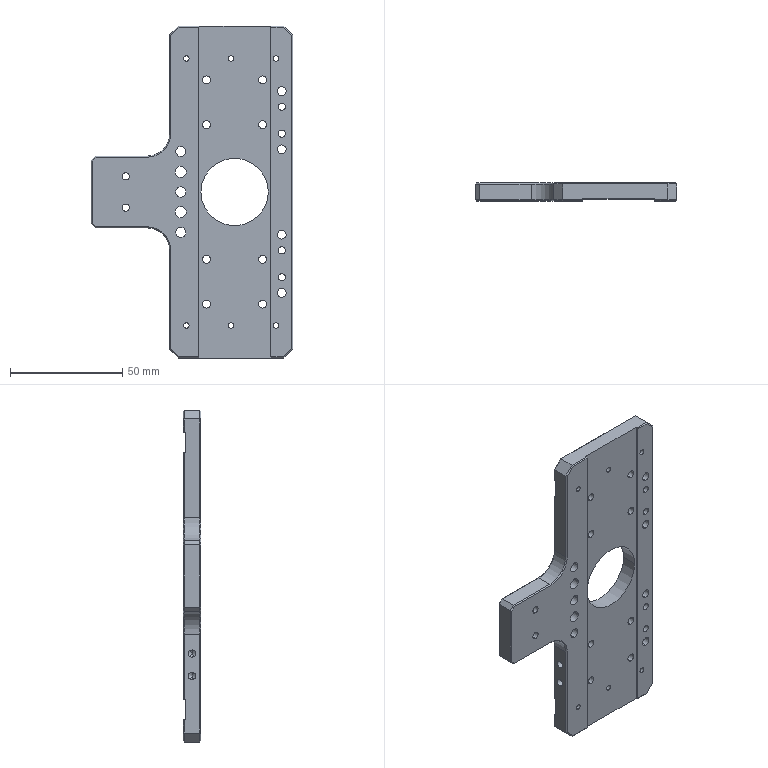Part | STEP file | A033 | 1 solid | 169 faces | box 90 x 8 x 148 mm | volume 59811 mm3 | cylinder 88 | plane 73 | cone 8 | commonest cylinder face diameters 3.5 x16 6.5 x16 2.459 x12 3.242 x12 4 x8 4.5 x6